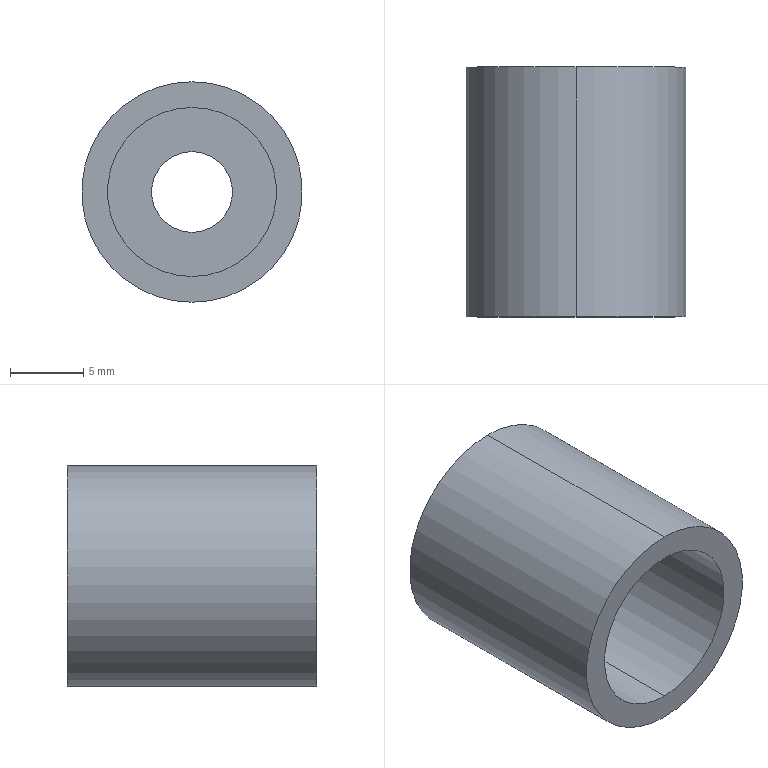Part | STEP file | countersunk screw spacer block | 1 solid | 9 faces | box 15 x 17 x 15 mm | volume 1639 mm3 | cylinder 6 | plane 3 | commonest cylinder face diameters 5.5 x2 11.5 x2 15 x2
STEP:
#1=CARTESIAN_POINT('',(0.,0.,0.));
#2=DIRECTION('',(0.,0.,1.));
#3=DIRECTION('',(1.,0.,0.));
#4=AXIS2_PLACEMENT_3D('',#1,#2,#3);
#5=CARTESIAN_POINT('',(0.,12.,-5.75));
#6=VERTEX_POINT('',#5);
#7=CARTESIAN_POINT('',(0.,0.,-5.75));
#8=VERTEX_POINT('',#7);
#9=CARTESIAN_POINT('',(0.,0.,-5.75));
#10=DIRECTION('',(0.,-1.,0.));
#11=VECTOR('',#10,1.);
#12=LINE('',#9,#11);
#13=CARTESIAN_POINT('',(0.,0.,0.));
#14=DIRECTION('',(0.,-1.,0.));
#15=DIRECTION('',(0.,0.,-1.));
#16=AXIS2_PLACEMENT_3D('',#13,#14,#15);
#17=CYLINDRICAL_SURFACE('',#16,5.75);
#18=CARTESIAN_POINT('',(6.283,0.));
#19=DIRECTION('',(0.,1.));
#20=VECTOR('',#19,1.);
#21=LINE('',#18,#20);
#22=(GEOMETRIC_REPRESENTATION_CONTEXT(2)PARAMETRIC_REPRESENTATION_CONTEXT()REPRESENTATION_CONTEXT('',''));
#23=DEFINITIONAL_REPRESENTATION('',(#21),#22);
#24=PCURVE('',#17,#23);
#25=CARTESIAN_POINT('',(0.,0.,0.));
#26=DIRECTION('',(0.,-1.,0.));
#27=DIRECTION('',(0.,0.,-1.));
#28=AXIS2_PLACEMENT_3D('',#25,#26,#27);
#29=CYLINDRICAL_SURFACE('',#28,5.75);
#30=CARTESIAN_POINT('',(0.,0.));
#31=DIRECTION('',(0.,1.));
#32=VECTOR('',#31,1.);
#33=LINE('',#30,#32);
#34=(GEOMETRIC_REPRESENTATION_CONTEXT(2)PARAMETRIC_REPRESENTATION_CONTEXT()REPRESENTATION_CONTEXT('',''));
#35=DEFINITIONAL_REPRESENTATION('',(#33),#34);
#36=PCURVE('',#29,#35);
#37=SURFACE_CURVE('',#12,(#24,#36),.PCURVE_S1.);
#38=EDGE_CURVE('',#6,#8,#37,.T.);
#39=ORIENTED_EDGE('',*,*,#38,.T.);
#40=CARTESIAN_POINT('',(0.,0.,5.75));
#41=VERTEX_POINT('',#40);
#42=CARTESIAN_POINT('',(0.,0.,0.));
#43=DIRECTION('',(0.,-1.,0.));
#44=DIRECTION('',(0.,0.,-1.));
#45=AXIS2_PLACEMENT_3D('',#42,#43,#44);
#46=CIRCLE('',#45,5.75);
#47=CARTESIAN_POINT('',(0.,0.));
#48=DIRECTION('',(1.,0.));
#49=VECTOR('',#48,1.);
#50=LINE('',#47,#49);
#51=(GEOMETRIC_REPRESENTATION_CONTEXT(2)PARAMETRIC_REPRESENTATION_CONTEXT()REPRESENTATION_CONTEXT('',''));
#52=DEFINITIONAL_REPRESENTATION('',(#50),#51);
#53=PCURVE('',#17,#52);
#54=CARTESIAN_POINT('',(0.,0.,0.));
#55=DIRECTION('',(0.,1.,0.));
#56=DIRECTION('',(0.,0.,1.));
#57=AXIS2_PLACEMENT_3D('',#54,#55,#56);
#58=PLANE('',#57);
#59=CARTESIAN_POINT('',(-5.75,0.));
#60=CARTESIAN_POINT('',(-5.75,9.959));
#61=CARTESIAN_POINT('',(2.875,4.98));
#62=CARTESIAN_POINT('',(11.5,0.));
#63=CARTESIAN_POINT('',(2.875,-4.98));
#64=CARTESIAN_POINT('',(-5.75,-9.959));
#65=CARTESIAN_POINT('',(-5.75,0.));
#66=(BOUNDED_CURVE()B_SPLINE_CURVE(2,(#59,#60,#61,#62,#63,#64,#65),.UNSPECIFIED.,.T.,.F.)B_SPLINE_CURVE_WITH_KNOTS((1,2,2,2,2,1),(-2.094,0.,2.094,4.189,6.283,8.378),.UNSPECIFIED.)CURVE()GEOMETRIC_REPRESENTATION_ITEM()RATIONAL_B_SPLINE_CURVE((1.,0.5,1.,0.5,1.,0.5,1.))REPRESENTATION_ITEM(''));
#67=(GEOMETRIC_REPRESENTATION_CONTEXT(2)PARAMETRIC_REPRESENTATION_CONTEXT()REPRESENTATION_CONTEXT('',''));
#68=DEFINITIONAL_REPRESENTATION('',(#66),#67);
#69=PCURVE('',#58,#68);
#70=SURFACE_CURVE('',#46,(#53,#69),.PCURVE_S1.);
#71=EDGE_CURVE('',#41,#8,#70,.T.);
#72=ORIENTED_EDGE('',*,*,#71,.F.);
#73=CARTESIAN_POINT('',(0.,12.,5.75));
#74=VERTEX_POINT('',#73);
#75=CARTESIAN_POINT('',(0.,0.,5.75));
#76=DIRECTION('',(0.,-1.,0.));
#77=VECTOR('',#76,1.);
#78=LINE('',#75,#77);
#79=CARTESIAN_POINT('',(3.142,0.));
#80=DIRECTION('',(0.,1.));
#81=VECTOR('',#80,1.);
#82=LINE('',#79,#81);
#83=(GEOMETRIC_REPRESENTATION_CONTEXT(2)PARAMETRIC_REPRESENTATION_CONTEXT()REPRESENTATION_CONTEXT('',''));
#84=DEFINITIONAL_REPRESENTATION('',(#82),#83);
#85=PCURVE('',#17,#84);
#86=CARTESIAN_POINT('',(3.142,0.));
#87=DIRECTION('',(0.,1.));
#88=VECTOR('',#87,1.);
#89=LINE('',#86,#88);
#90=(GEOMETRIC_REPRESENTATION_CONTEXT(2)PARAMETRIC_REPRESENTATION_CONTEXT()REPRESENTATION_CONTEXT('',''));
#91=DEFINITIONAL_REPRESENTATION('',(#89),#90);
#92=PCURVE('',#29,#91);
#93=SURFACE_CURVE('',#78,(#85,#92),.PCURVE_S1.);
#94=EDGE_CURVE('',#74,#41,#93,.T.);
#95=ORIENTED_EDGE('',*,*,#94,.F.);
#96=CARTESIAN_POINT('',(0.,12.,0.));
#97=DIRECTION('',(0.,-1.,0.));
#98=DIRECTION('',(0.,0.,-1.));
#99=AXIS2_PLACEMENT_3D('',#96,#97,#98);
#100=CIRCLE('',#99,5.75);
#101=CARTESIAN_POINT('',(0.,-12.));
#102=DIRECTION('',(1.,0.));
#103=VECTOR('',#102,1.);
#104=LINE('',#101,#103);
#105=(GEOMETRIC_REPRESENTATION_CONTEXT(2)PARAMETRIC_REPRESENTATION_CONTEXT()REPRESENTATION_CONTEXT('',''));
#106=DEFINITIONAL_REPRESENTATION('',(#104),#105);
#107=PCURVE('',#17,#106);
#108=CARTESIAN_POINT('',(2.75,12.,0.));
#109=DIRECTION('',(0.,1.,0.));
#110=DIRECTION('',(0.,0.,1.));
#111=AXIS2_PLACEMENT_3D('',#108,#109,#110);
#112=PLANE('',#111);
#113=CARTESIAN_POINT('',(-5.75,-2.75));
#114=CARTESIAN_POINT('',(-5.75,7.209));
#115=CARTESIAN_POINT('',(2.875,2.23));
#116=CARTESIAN_POINT('',(11.5,-2.75));
#117=CARTESIAN_POINT('',(2.875,-7.73));
#118=CARTESIAN_POINT('',(-5.75,-12.709));
#119=CARTESIAN_POINT('',(-5.75,-2.75));
#120=(BOUNDED_CURVE()B_SPLINE_CURVE(2,(#113,#114,#115,#116,#117,#118,#119),.UNSPECIFIED.,.T.,.F.)B_SPLINE_CURVE_WITH_KNOTS((1,2,2,2,2,1),(-2.094,0.,2.094,4.189,6.283,8.378),.UNSPECIFIED.)CURVE()GEOMETRIC_REPRESENTATION_ITEM()RATIONAL_B_SPLINE_CURVE((1.,0.5,1.,0.5,1.,0.5,1.))REPRESENTATION_ITEM(''));
#121=(GEOMETRIC_REPRESENTATION_CONTEXT(2)PARAMETRIC_REPRESENTATION_CONTEXT()REPRESENTATION_CONTEXT('',''));
#122=DEFINITIONAL_REPRESENTATION('',(#120),#121);
#123=PCURVE('',#112,#122);
#124=SURFACE_CURVE('',#100,(#107,#123),.PCURVE_S1.);
#125=EDGE_CURVE('',#74,#6,#124,.T.);
#126=ORIENTED_EDGE('',*,*,#125,.T.);
#127=EDGE_LOOP('',(#39,#72,#95,#126));
#128=FACE_BOUND('',#127,.F.);
#129=ADVANCED_FACE('',(#128),#17,.F.);
#130=CARTESIAN_POINT('',(0.,17.,-2.75));
#131=VERTEX_POINT('',#130);
#132=CARTESIAN_POINT('',(0.,12.,-2.75));
#133=VERTEX_POINT('',#132);
#134=CARTESIAN_POINT('',(0.,0.,-2.75));
#135=DIRECTION('',(0.,-1.,0.));
#136=VECTOR('',#135,1.);
#137=LINE('',#134,#136);
#138=CARTESIAN_POINT('',(0.,0.,0.));
#139=DIRECTION('',(0.,-1.,0.));
#140=DIRECTION('',(0.,0.,-1.));
#141=AXIS2_PLACEMENT_3D('',#138,#139,#140);
#142=CYLINDRICAL_SURFACE('',#141,2.75);
#143=CARTESIAN_POINT('',(6.283,0.));
#144=DIRECTION('',(0.,1.));
#145=VECTOR('',#144,1.);
#146=LINE('',#143,#145);
#147=(GEOMETRIC_REPRESENTATION_CONTEXT(2)PARAMETRIC_REPRESENTATION_CONTEXT()REPRESENTATION_CONTEXT('',''));
#148=DEFINITIONAL_REPRESENTATION('',(#146),#147);
#149=PCURVE('',#142,#148);
#150=CARTESIAN_POINT('',(0.,0.,0.));
#151=DIRECTION('',(0.,-1.,0.));
#152=DIRECTION('',(0.,0.,-1.));
#153=AXIS2_PLACEMENT_3D('',#150,#151,#152);
#154=CYLINDRICAL_SURFACE('',#153,2.75);
#155=CARTESIAN_POINT('',(0.,0.));
#156=DIRECTION('',(0.,1.));
#157=VECTOR('',#156,1.);
#158=LINE('',#155,#157);
#159=(GEOMETRIC_REPRESENTATION_CONTEXT(2)PARAMETRIC_REPRESENTATION_CONTEXT()REPRESENTATION_CONTEXT('',''));
#160=DEFINITIONAL_REPRESENTATION('',(#158),#159);
#161=PCURVE('',#154,#160);
#162=SURFACE_CURVE('',#137,(#149,#161),.PCURVE_S1.);
#163=EDGE_CURVE('',#131,#133,#162,.T.);
#164=ORIENTED_EDGE('',*,*,#163,.T.);
#165=CARTESIAN_POINT('',(0.,12.,2.75));
#166=VERTEX_POINT('',#165);
#167=CARTESIAN_POINT('',(0.,12.,0.));
#168=DIRECTION('',(0.,-1.,0.));
#169=DIRECTION('',(0.,0.,-1.));
#170=AXIS2_PLACEMENT_3D('',#167,#168,#169);
#171=CIRCLE('',#170,2.75);
#172=CARTESIAN_POINT('',(0.,-12.));
#173=DIRECTION('',(1.,0.));
#174=VECTOR('',#173,1.);
#175=LINE('',#172,#174);
#176=(GEOMETRIC_REPRESENTATION_CONTEXT(2)PARAMETRIC_REPRESENTATION_CONTEXT()REPRESENTATION_CONTEXT('',''));
#177=DEFINITIONAL_REPRESENTATION('',(#175),#176);
#178=PCURVE('',#142,#177);
#179=CARTESIAN_POINT('',(-2.75,-2.75));
#180=CARTESIAN_POINT('',(-2.75,2.013));
#181=CARTESIAN_POINT('',(1.375,-0.3684));
#182=CARTESIAN_POINT('',(5.5,-2.75));
#183=CARTESIAN_POINT('',(1.375,-5.132));
#184=CARTESIAN_POINT('',(-2.75,-7.513));
#185=CARTESIAN_POINT('',(-2.75,-2.75));
#186=(BOUNDED_CURVE()B_SPLINE_CURVE(2,(#179,#180,#181,#182,#183,#184,#185),.UNSPECIFIED.,.T.,.F.)B_SPLINE_CURVE_WITH_KNOTS((1,2,2,2,2,1),(-2.094,0.,2.094,4.189,6.283,8.378),.UNSPECIFIED.)CURVE()GEOMETRIC_REPRESENTATION_ITEM()RATIONAL_B_SPLINE_CURVE((1.,0.5,1.,0.5,1.,0.5,1.))REPRESENTATION_ITEM(''));
#187=(GEOMETRIC_REPRESENTATION_CONTEXT(2)PARAMETRIC_REPRESENTATION_CONTEXT()REPRESENTATION_CONTEXT('',''));
#188=DEFINITIONAL_REPRESENTATION('',(#186),#187);
#189=PCURVE('',#112,#188);
#190=SURFACE_CURVE('',#171,(#178,#189),.PCURVE_S1.);
#191=EDGE_CURVE('',#166,#133,#190,.T.);
#192=ORIENTED_EDGE('',*,*,#191,.F.);
#193=CARTESIAN_POINT('',(0.,17.,2.75));
#194=VERTEX_POINT('',#193);
#195=CARTESIAN_POINT('',(0.,0.,2.75));
#196=DIRECTION('',(0.,-1.,0.));
#197=VECTOR('',#196,1.);
#198=LINE('',#195,#197);
#199=CARTESIAN_POINT('',(3.142,0.));
#200=DIRECTION('',(0.,1.));
#201=VECTOR('',#200,1.);
#202=LINE('',#199,#201);
#203=(GEOMETRIC_REPRESENTATION_CONTEXT(2)PARAMETRIC_REPRESENTATION_CONTEXT()REPRESENTATION_CONTEXT('',''));
#204=DEFINITIONAL_REPRESENTATION('',(#202),#203);
#205=PCURVE('',#142,#204);
#206=CARTESIAN_POINT('',(3.142,0.));
#207=DIRECTION('',(0.,1.));
#208=VECTOR('',#207,1.);
#209=LINE('',#206,#208);
#210=(GEOMETRIC_REPRESENTATION_CONTEXT(2)PARAMETRIC_REPRESENTATION_CONTEXT()REPRESENTATION_CONTEXT('',''));
#211=DEFINITIONAL_REPRESENTATION('',(#209),#210);
#212=PCURVE('',#154,#211);
#213=SURFACE_CURVE('',#198,(#205,#212),.PCURVE_S1.);
#214=EDGE_CURVE('',#194,#166,#213,.T.);
#215=ORIENTED_EDGE('',*,*,#214,.F.);
#216=CARTESIAN_POINT('',(0.,17.,0.));
#217=DIRECTION('',(0.,-1.,0.));
#218=DIRECTION('',(0.,0.,-1.));
#219=AXIS2_PLACEMENT_3D('',#216,#217,#218);
#220=CIRCLE('',#219,2.75);
#221=CARTESIAN_POINT('',(0.,-17.));
#222=DIRECTION('',(1.,0.));
#223=VECTOR('',#222,1.);
#224=LINE('',#221,#223);
#225=(GEOMETRIC_REPRESENTATION_CONTEXT(2)PARAMETRIC_REPRESENTATION_CONTEXT()REPRESENTATION_CONTEXT('',''));
#226=DEFINITIONAL_REPRESENTATION('',(#224),#225);
#227=PCURVE('',#142,#226);
#228=CARTESIAN_POINT('',(0.,17.,0.));
#229=DIRECTION('',(0.,1.,0.));
#230=DIRECTION('',(0.,0.,1.));
#231=AXIS2_PLACEMENT_3D('',#228,#229,#230);
#232=PLANE('',#231);
#233=CARTESIAN_POINT('',(-2.75,0.));
#234=CARTESIAN_POINT('',(-2.75,4.763));
#235=CARTESIAN_POINT('',(1.375,2.382));
#236=CARTESIAN_POINT('',(5.5,0.));
#237=CARTESIAN_POINT('',(1.375,-2.382));
#238=CARTESIAN_POINT('',(-2.75,-4.763));
#239=CARTESIAN_POINT('',(-2.75,0.));
#240=(BOUNDED_CURVE()B_SPLINE_CURVE(2,(#233,#234,#235,#236,#237,#238,#239),.UNSPECIFIED.,.T.,.F.)B_SPLINE_CURVE_WITH_KNOTS((1,2,2,2,2,1),(-2.094,0.,2.094,4.189,6.283,8.378),.UNSPECIFIED.)CURVE()GEOMETRIC_REPRESENTATION_ITEM()RATIONAL_B_SPLINE_CURVE((1.,0.5,1.,0.5,1.,0.5,1.))REPRESENTATION_ITEM(''));
#241=(GEOMETRIC_REPRESENTATION_CONTEXT(2)PARAMETRIC_REPRESENTATION_CONTEXT()REPRESENTATION_CONTEXT('',''));
#242=DEFINITIONAL_REPRESENTATION('',(#240),#241);
#243=PCURVE('',#232,#242);
#244=SURFACE_CURVE('',#220,(#227,#243),.PCURVE_S1.);
#245=EDGE_CURVE('',#194,#131,#244,.T.);
#246=ORIENTED_EDGE('',*,*,#245,.T.);
#247=EDGE_LOOP('',(#164,#192,#215,#246));
#248=FACE_BOUND('',#247,.F.);
#249=ADVANCED_FACE('',(#248),#142,.F.);
#250=CARTESIAN_POINT('',(0.,17.,7.5));
#251=VERTEX_POINT('',#250);
#252=CARTESIAN_POINT('',(0.,17.,-7.5));
#253=VERTEX_POINT('',#252);
#254=CARTESIAN_POINT('',(0.,17.,0.));
#255=DIRECTION('',(0.,1.,0.));
#256=DIRECTION('',(0.,0.,1.));
#257=AXIS2_PLACEMENT_3D('',#254,#255,#256);
#258=CIRCLE('',#257,7.5);
#259=CARTESIAN_POINT('',(0.,17.,0.));
#260=DIRECTION('',(0.,-1.,0.));
#261=DIRECTION('',(0.,0.,-1.));
#262=AXIS2_PLACEMENT_3D('',#259,#260,#261);
#263=CYLINDRICAL_SURFACE('',#262,7.5);
#264=CARTESIAN_POINT('',(3.142,0.));
#265=DIRECTION('',(-1.,0.));
#266=VECTOR('',#265,1.);
#267=LINE('',#264,#266);
#268=(GEOMETRIC_REPRESENTATION_CONTEXT(2)PARAMETRIC_REPRESENTATION_CONTEXT()REPRESENTATION_CONTEXT('',''));
#269=DEFINITIONAL_REPRESENTATION('',(#267),#268);
#270=PCURVE('',#263,#269);
#271=CARTESIAN_POINT('',(0.,0.));
#272=DIRECTION('',(1.,0.));
#273=AXIS2_PLACEMENT_2D('',#271,#272);
#274=CIRCLE('',#273,7.5);
#275=(GEOMETRIC_REPRESENTATION_CONTEXT(2)PARAMETRIC_REPRESENTATION_CONTEXT()REPRESENTATION_CONTEXT('',''));
#276=DEFINITIONAL_REPRESENTATION('',(#274),#275);
#277=PCURVE('',#232,#276);
#278=SURFACE_CURVE('',#258,(#270,#277),.PCURVE_S1.);
#279=EDGE_CURVE('',#251,#253,#278,.T.);
#280=ORIENTED_EDGE('',*,*,#279,.F.);
#281=CARTESIAN_POINT('',(0.,0.,7.5));
#282=VERTEX_POINT('',#281);
#283=CARTESIAN_POINT('',(0.,17.,7.5));
#284=DIRECTION('',(0.,-1.,0.));
#285=VECTOR('',#284,1.);
#286=LINE('',#283,#285);
#287=CARTESIAN_POINT('',(3.142,0.));
#288=DIRECTION('',(0.,1.));
#289=VECTOR('',#288,1.);
#290=LINE('',#287,#289);
#291=(GEOMETRIC_REPRESENTATION_CONTEXT(2)PARAMETRIC_REPRESENTATION_CONTEXT()REPRESENTATION_CONTEXT('',''));
#292=DEFINITIONAL_REPRESENTATION('',(#290),#291);
#293=PCURVE('',#263,#292);
#294=CARTESIAN_POINT('',(0.,17.,0.));
#295=DIRECTION('',(0.,-1.,0.));
#296=DIRECTION('',(0.,0.,-1.));
#297=AXIS2_PLACEMENT_3D('',#294,#295,#296);
#298=CYLINDRICAL_SURFACE('',#297,7.5);
#299=CARTESIAN_POINT('',(3.142,0.));
#300=DIRECTION('',(0.,1.));
#301=VECTOR('',#300,1.);
#302=LINE('',#299,#301);
#303=(GEOMETRIC_REPRESENTATION_CONTEXT(2)PARAMETRIC_REPRESENTATION_CONTEXT()REPRESENTATION_CONTEXT('',''));
#304=DEFINITIONAL_REPRESENTATION('',(#302),#303);
#305=PCURVE('',#298,#304);
#306=SURFACE_CURVE('',#286,(#293,#305),.PCURVE_S1.);
#307=EDGE_CURVE('',#251,#282,#306,.T.);
#308=ORIENTED_EDGE('',*,*,#307,.T.);
#309=CARTESIAN_POINT('',(0.,0.,-7.5));
#310=VERTEX_POINT('',#309);
#311=CARTESIAN_POINT('',(0.,0.,0.));
#312=DIRECTION('',(0.,1.,0.));
#313=DIRECTION('',(0.,0.,1.));
#314=AXIS2_PLACEMENT_3D('',#311,#312,#313);
#315=CIRCLE('',#314,7.5);
#316=CARTESIAN_POINT('',(3.142,17.));
#317=DIRECTION('',(-1.,0.));
#318=VECTOR('',#317,1.);
#319=LINE('',#316,#318);
#320=(GEOMETRIC_REPRESENTATION_CONTEXT(2)PARAMETRIC_REPRESENTATION_CONTEXT()REPRESENTATION_CONTEXT('',''));
#321=DEFINITIONAL_REPRESENTATION('',(#319),#320);
#322=PCURVE('',#263,#321);
#323=CARTESIAN_POINT('',(0.,0.));
#324=DIRECTION('',(1.,0.));
#325=AXIS2_PLACEMENT_2D('',#323,#324);
#326=CIRCLE('',#325,7.5);
#327=(GEOMETRIC_REPRESENTATION_CONTEXT(2)PARAMETRIC_REPRESENTATION_CONTEXT()REPRESENTATION_CONTEXT('',''));
#328=DEFINITIONAL_REPRESENTATION('',(#326),#327);
#329=PCURVE('',#58,#328);
#330=SURFACE_CURVE('',#315,(#322,#329),.PCURVE_S1.);
#331=EDGE_CURVE('',#282,#310,#330,.T.);
#332=ORIENTED_EDGE('',*,*,#331,.T.);
#333=CARTESIAN_POINT('',(0.,17.,-7.5));
#334=DIRECTION('',(0.,-1.,0.));
#335=VECTOR('',#334,1.);
#336=LINE('',#333,#335);
#337=CARTESIAN_POINT('',(0.,0.));
#338=DIRECTION('',(0.,1.));
#339=VECTOR('',#338,1.);
#340=LINE('',#337,#339);
#341=(GEOMETRIC_REPRESENTATION_CONTEXT(2)PARAMETRIC_REPRESENTATION_CONTEXT()REPRESENTATION_CONTEXT('',''));
#342=DEFINITIONAL_REPRESENTATION('',(#340),#341);
#343=PCURVE('',#263,#342);
#344=CARTESIAN_POINT('',(6.283,0.));
#345=DIRECTION('',(0.,1.));
#346=VECTOR('',#345,1.);
#347=LINE('',#344,#346);
#348=(GEOMETRIC_REPRESENTATION_CONTEXT(2)PARAMETRIC_REPRESENTATION_CONTEXT()REPRESENTATION_CONTEXT('',''));
#349=DEFINITIONAL_REPRESENTATION('',(#347),#348);
#350=PCURVE('',#298,#349);
#351=SURFACE_CURVE('',#336,(#343,#350),.PCURVE_S1.);
#352=EDGE_CURVE('',#253,#310,#351,.T.);
#353=ORIENTED_EDGE('',*,*,#352,.F.);
#354=EDGE_LOOP('',(#280,#308,#332,#353));
#355=FACE_BOUND('',#354,.T.);
#356=ADVANCED_FACE('',(#355),#263,.T.);
#357=ORIENTED_EDGE('',*,*,#307,.F.);
#358=CARTESIAN_POINT('',(0.,17.,0.));
#359=DIRECTION('',(0.,1.,0.));
#360=DIRECTION('',(0.,0.,1.));
#361=AXIS2_PLACEMENT_3D('',#358,#359,#360);
#362=CIRCLE('',#361,7.5);
#363=CARTESIAN_POINT('',(9.425,0.));
#364=DIRECTION('',(-1.,0.));
#365=VECTOR('',#364,1.);
#366=LINE('',#363,#365);
#367=(GEOMETRIC_REPRESENTATION_CONTEXT(2)PARAMETRIC_REPRESENTATION_CONTEXT()REPRESENTATION_CONTEXT('',''));
#368=DEFINITIONAL_REPRESENTATION('',(#366),#367);
#369=PCURVE('',#298,#368);
#370=CARTESIAN_POINT('',(0.,0.));
#371=DIRECTION('',(1.,0.));
#372=AXIS2_PLACEMENT_2D('',#370,#371);
#373=CIRCLE('',#372,7.5);
#374=(GEOMETRIC_REPRESENTATION_CONTEXT(2)PARAMETRIC_REPRESENTATION_CONTEXT()REPRESENTATION_CONTEXT('',''));
#375=DEFINITIONAL_REPRESENTATION('',(#373),#374);
#376=PCURVE('',#232,#375);
#377=SURFACE_CURVE('',#362,(#369,#376),.PCURVE_S1.);
#378=EDGE_CURVE('',#253,#251,#377,.T.);
#379=ORIENTED_EDGE('',*,*,#378,.F.);
#380=ORIENTED_EDGE('',*,*,#352,.T.);
#381=CARTESIAN_POINT('',(0.,0.,0.));
#382=DIRECTION('',(0.,1.,0.));
#383=DIRECTION('',(0.,0.,1.));
#384=AXIS2_PLACEMENT_3D('',#381,#382,#383);
#385=CIRCLE('',#384,7.5);
#386=CARTESIAN_POINT('',(9.425,17.));
#387=DIRECTION('',(-1.,0.));
#388=VECTOR('',#387,1.);
#389=LINE('',#386,#388);
#390=(GEOMETRIC_REPRESENTATION_CONTEXT(2)PARAMETRIC_REPRESENTATION_CONTEXT()REPRESENTATION_CONTEXT('',''));
#391=DEFINITIONAL_REPRESENTATION('',(#389),#390);
#392=PCURVE('',#298,#391);
#393=CARTESIAN_POINT('',(0.,0.));
#394=DIRECTION('',(1.,0.));
#395=AXIS2_PLACEMENT_2D('',#393,#394);
#396=CIRCLE('',#395,7.5);
#397=(GEOMETRIC_REPRESENTATION_CONTEXT(2)PARAMETRIC_REPRESENTATION_CONTEXT()REPRESENTATION_CONTEXT('',''));
#398=DEFINITIONAL_REPRESENTATION('',(#396),#397);
#399=PCURVE('',#58,#398);
#400=SURFACE_CURVE('',#385,(#392,#399),.PCURVE_S1.);
#401=EDGE_CURVE('',#310,#282,#400,.T.);
#402=ORIENTED_EDGE('',*,*,#401,.T.);
#403=EDGE_LOOP('',(#357,#379,#380,#402));
#404=FACE_BOUND('',#403,.T.);
#405=ADVANCED_FACE('',(#404),#298,.T.);
#406=CARTESIAN_POINT('',(0.,17.,0.));
#407=DIRECTION('',(0.,-1.,0.));
#408=DIRECTION('',(0.,0.,-1.));
#409=AXIS2_PLACEMENT_3D('',#406,#407,#408);
#410=CIRCLE('',#409,2.75);
#411=CARTESIAN_POINT('',(-2.75,0.));
#412=CARTESIAN_POINT('',(-2.75,4.763));
#413=CARTESIAN_POINT('',(1.375,2.382));
#414=CARTESIAN_POINT('',(5.5,0.));
#415=CARTESIAN_POINT('',(1.375,-2.382));
#416=CARTESIAN_POINT('',(-2.75,-4.763));
#417=CARTESIAN_POINT('',(-2.75,0.));
#418=(BOUNDED_CURVE()B_SPLINE_CURVE(2,(#411,#412,#413,#414,#415,#416,#417),.UNSPECIFIED.,.T.,.F.)B_SPLINE_CURVE_WITH_KNOTS((1,2,2,2,2,1),(-2.094,0.,2.094,4.189,6.283,8.378),.UNSPECIFIED.)CURVE()GEOMETRIC_REPRESENTATION_ITEM()RATIONAL_B_SPLINE_CURVE((1.,0.5,1.,0.5,1.,0.5,1.))REPRESENTATION_ITEM(''));
#419=(GEOMETRIC_REPRESENTATION_CONTEXT(2)PARAMETRIC_REPRESENTATION_CONTEXT()REPRESENTATION_CONTEXT('',''));
#420=DEFINITIONAL_REPRESENTATION('',(#418),#419);
#421=PCURVE('',#232,#420);
#422=CARTESIAN_POINT('',(0.,-17.));
#423=DIRECTION('',(1.,0.));
#424=VECTOR('',#423,1.);
#425=LINE('',#422,#424);
#426=(GEOMETRIC_REPRESENTATION_CONTEXT(2)PARAMETRIC_REPRESENTATION_CONTEXT()REPRESENTATION_CONTEXT('',''));
#427=DEFINITIONAL_REPRESENTATION('',(#425),#426);
#428=PCURVE('',#154,#427);
#429=SURFACE_CURVE('',#410,(#421,#428),.PCURVE_S1.);
#430=EDGE_CURVE('',#131,#194,#429,.T.);
#431=ORIENTED_EDGE('',*,*,#430,.T.);
#432=ORIENTED_EDGE('',*,*,#245,.T.);
#433=EDGE_LOOP('',(#431,#432));
#434=FACE_BOUND('',#433,.T.);
#435=ORIENTED_EDGE('',*,*,#378,.T.);
#436=ORIENTED_EDGE('',*,*,#279,.T.);
#437=EDGE_LOOP('',(#435,#436));
#438=FACE_BOUND('',#437,.T.);
#439=ADVANCED_FACE('',(#434,#438),#232,.T.);
#440=CARTESIAN_POINT('',(0.,0.,0.));
#441=DIRECTION('',(0.,-1.,0.));
#442=DIRECTION('',(0.,0.,-1.));
#443=AXIS2_PLACEMENT_3D('',#440,#441,#442);
#444=CIRCLE('',#443,5.75);
#445=CARTESIAN_POINT('',(-5.75,0.));
#446=CARTESIAN_POINT('',(-5.75,9.959));
#447=CARTESIAN_POINT('',(2.875,4.98));
#448=CARTESIAN_POINT('',(11.5,0.));
#449=CARTESIAN_POINT('',(2.875,-4.98));
#450=CARTESIAN_POINT('',(-5.75,-9.959));
#451=CARTESIAN_POINT('',(-5.75,0.));
#452=(BOUNDED_CURVE()B_SPLINE_CURVE(2,(#445,#446,#447,#448,#449,#450,#451),.UNSPECIFIED.,.T.,.F.)B_SPLINE_CURVE_WITH_KNOTS((1,2,2,2,2,1),(-2.094,0.,2.094,4.189,6.283,8.378),.UNSPECIFIED.)CURVE()GEOMETRIC_REPRESENTATION_ITEM()RATIONAL_B_SPLINE_CURVE((1.,0.5,1.,0.5,1.,0.5,1.))REPRESENTATION_ITEM(''));
#453=(GEOMETRIC_REPRESENTATION_CONTEXT(2)PARAMETRIC_REPRESENTATION_CONTEXT()REPRESENTATION_CONTEXT('',''));
#454=DEFINITIONAL_REPRESENTATION('',(#452),#453);
#455=PCURVE('',#58,#454);
#456=CARTESIAN_POINT('',(0.,0.));
#457=DIRECTION('',(1.,0.));
#458=VECTOR('',#457,1.);
#459=LINE('',#456,#458);
#460=(GEOMETRIC_REPRESENTATION_CONTEXT(2)PARAMETRIC_REPRESENTATION_CONTEXT()REPRESENTATION_CONTEXT('',''));
#461=DEFINITIONAL_REPRESENTATION('',(#459),#460);
#462=PCURVE('',#29,#461);
#463=SURFACE_CURVE('',#444,(#455,#462),.PCURVE_S1.);
#464=EDGE_CURVE('',#8,#41,#463,.T.);
#465=ORIENTED_EDGE('',*,*,#464,.F.);
#466=ORIENTED_EDGE('',*,*,#71,.F.);
#467=EDGE_LOOP('',(#465,#466));
#468=FACE_BOUND('',#467,.T.);
#469=ORIENTED_EDGE('',*,*,#401,.F.);
#470=ORIENTED_EDGE('',*,*,#331,.F.);
#471=EDGE_LOOP('',(#469,#470));
#472=FACE_BOUND('',#471,.T.);
#473=ADVANCED_FACE('',(#468,#472),#58,.F.);
#474=CARTESIAN_POINT('',(0.,12.,0.));
#475=DIRECTION('',(0.,-1.,0.));
#476=DIRECTION('',(0.,0.,-1.));
#477=AXIS2_PLACEMENT_3D('',#474,#475,#476);
#478=CIRCLE('',#477,2.75);
#479=CARTESIAN_POINT('',(0.,-12.));
#480=DIRECTION('',(1.,0.));
#481=VECTOR('',#480,1.);
#482=LINE('',#479,#481);
#483=(GEOMETRIC_REPRESENTATION_CONTEXT(2)PARAMETRIC_REPRESENTATION_CONTEXT()REPRESENTATION_CONTEXT('',''));
#484=DEFINITIONAL_REPRESENTATION('',(#482),#483);
#485=PCURVE('',#154,#484);
#486=CARTESIAN_POINT('',(-2.75,-2.75));
#487=CARTESIAN_POINT('',(-2.75,2.013));
#488=CARTESIAN_POINT('',(1.375,-0.3684));
#489=CARTESIAN_POINT('',(5.5,-2.75));
#490=CARTESIAN_POINT('',(1.375,-5.132));
#491=CARTESIAN_POINT('',(-2.75,-7.513));
#492=CARTESIAN_POINT('',(-2.75,-2.75));
#493=(BOUNDED_CURVE()B_SPLINE_CURVE(2,(#486,#487,#488,#489,#490,#491,#492),.UNSPECIFIED.,.T.,.F.)B_SPLINE_CURVE_WITH_KNOTS((1,2,2,2,2,1),(-2.094,0.,2.094,4.189,6.283,8.378),.UNSPECIFIED.)CURVE()GEOMETRIC_REPRESENTATION_ITEM()RATIONAL_B_SPLINE_CURVE((1.,0.5,1.,0.5,1.,0.5,1.))REPRESENTATION_ITEM(''));
#494=(GEOMETRIC_REPRESENTATION_CONTEXT(2)PARAMETRIC_REPRESENTATION_CONTEXT()REPRESENTATION_CONTEXT('',''));
#495=DEFINITIONAL_REPRESENTATION('',(#493),#494);
#496=PCURVE('',#112,#495);
#497=SURFACE_CURVE('',#478,(#485,#496),.PCURVE_S1.);
#498=EDGE_CURVE('',#133,#166,#497,.T.);
#499=ORIENTED_EDGE('',*,*,#498,.F.);
#500=ORIENTED_EDGE('',*,*,#163,.F.);
#501=ORIENTED_EDGE('',*,*,#430,.T.);
#502=ORIENTED_EDGE('',*,*,#214,.T.);
#503=EDGE_LOOP('',(#499,#500,#501,#502));
#504=FACE_BOUND('',#503,.F.);
#505=ADVANCED_FACE('',(#504),#154,.F.);
#506=ORIENTED_EDGE('',*,*,#498,.F.);
#507=ORIENTED_EDGE('',*,*,#191,.F.);
#508=EDGE_LOOP('',(#506,#507));
#509=FACE_BOUND('',#508,.T.);
#510=CARTESIAN_POINT('',(0.,12.,0.));
#511=DIRECTION('',(0.,-1.,0.));
#512=DIRECTION('',(0.,0.,-1.));
#513=AXIS2_PLACEMENT_3D('',#510,#511,#512);
#514=CIRCLE('',#513,5.75);
#515=CARTESIAN_POINT('',(-5.75,-2.75));
#516=CARTESIAN_POINT('',(-5.75,7.209));
#517=CARTESIAN_POINT('',(2.875,2.23));
#518=CARTESIAN_POINT('',(11.5,-2.75));
#519=CARTESIAN_POINT('',(2.875,-7.73));
#520=CARTESIAN_POINT('',(-5.75,-12.709));
#521=CARTESIAN_POINT('',(-5.75,-2.75));
#522=(BOUNDED_CURVE()B_SPLINE_CURVE(2,(#515,#516,#517,#518,#519,#520,#521),.UNSPECIFIED.,.T.,.F.)B_SPLINE_CURVE_WITH_KNOTS((1,2,2,2,2,1),(-2.094,0.,2.094,4.189,6.283,8.378),.UNSPECIFIED.)CURVE()GEOMETRIC_REPRESENTATION_ITEM()RATIONAL_B_SPLINE_CURVE((1.,0.5,1.,0.5,1.,0.5,1.))REPRESENTATION_ITEM(''));
#523=(GEOMETRIC_REPRESENTATION_CONTEXT(2)PARAMETRIC_REPRESENTATION_CONTEXT()REPRESENTATION_CONTEXT('',''));
#524=DEFINITIONAL_REPRESENTATION('',(#522),#523);
#525=PCURVE('',#112,#524);
#526=CARTESIAN_POINT('',(0.,-12.));
#527=DIRECTION('',(1.,0.));
#528=VECTOR('',#527,1.);
#529=LINE('',#526,#528);
#530=(GEOMETRIC_REPRESENTATION_CONTEXT(2)PARAMETRIC_REPRESENTATION_CONTEXT()REPRESENTATION_CONTEXT('',''));
#531=DEFINITIONAL_REPRESENTATION('',(#529),#530);
#532=PCURVE('',#29,#531);
#533=SURFACE_CURVE('',#514,(#525,#532),.PCURVE_S1.);
#534=EDGE_CURVE('',#6,#74,#533,.T.);
#535=ORIENTED_EDGE('',*,*,#534,.T.);
#536=ORIENTED_EDGE('',*,*,#125,.T.);
#537=EDGE_LOOP('',(#535,#536));
#538=FACE_BOUND('',#537,.T.);
#539=ADVANCED_FACE('',(#509,#538),#112,.F.);
#540=ORIENTED_EDGE('',*,*,#464,.F.);
#541=ORIENTED_EDGE('',*,*,#38,.F.);
#542=ORIENTED_EDGE('',*,*,#534,.T.);
#543=ORIENTED_EDGE('',*,*,#94,.T.);
#544=EDGE_LOOP('',(#540,#541,#542,#543));
#545=FACE_BOUND('',#544,.F.);
#546=ADVANCED_FACE('',(#545),#29,.F.);
#547=CLOSED_SHELL('',(#129,#249,#356,#405,#439,#473,#505,#539,#546));
#548=MANIFOLD_SOLID_BREP('',#547);
#549=(LENGTH_UNIT()NAMED_UNIT(*)SI_UNIT(.MILLI.,.METRE.));
#550=UNCERTAINTY_MEASURE_WITH_UNIT(LENGTH_MEASURE(0.0000001),#549,'','');
#551=(NAMED_UNIT(*)PLANE_ANGLE_UNIT()SI_UNIT($,.RADIAN.));
#552=(NAMED_UNIT(*)SI_UNIT($,.STERADIAN.)SOLID_ANGLE_UNIT());
#553=(GEOMETRIC_REPRESENTATION_CONTEXT(3)GLOBAL_UNCERTAINTY_ASSIGNED_CONTEXT((#550))GLOBAL_UNIT_ASSIGNED_CONTEXT((#549,#551,#552))REPRESENTATION_CONTEXT('',''));
#554=ADVANCED_BREP_SHAPE_REPRESENTATION('',(#4,#548),#553);